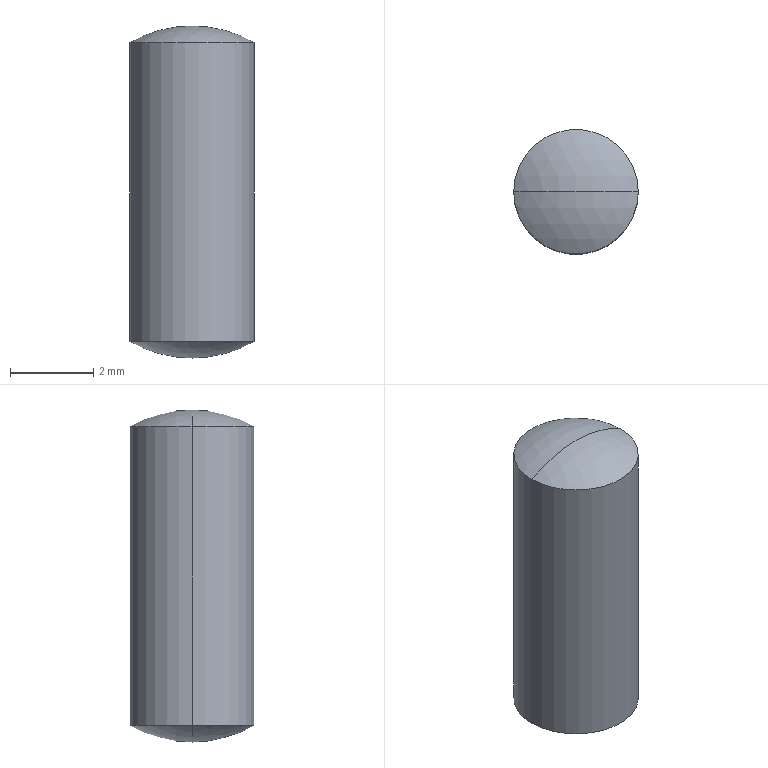Part | SolidWorks | features Attribute 1, Revolution 1 | 1 solid | 6 faces | box 3 x 3 x 8 mm | volume 53.776 mm3 | sphere 4 | cylinder 2 | commonest cylinder face diameters 3 x2
STEP:
#1=CARTESIAN_POINT('',(-1.5,0.,1.598));
#2=VERTEX_POINT('',#1);
#3=CARTESIAN_POINT('',(1.5,0.,1.598));
#4=VERTEX_POINT('',#3);
#5=CARTESIAN_POINT('',(0.,0.,1.598));
#6=DIRECTION('',(0.,0.,-1.));
#7=DIRECTION('',(-1.,0.,0.));
#8=AXIS2_PLACEMENT_3D('',#5,#6,#7);
#9=CIRCLE('',#8,1.5);
#10=EDGE_CURVE('',#2,#4,#9,.T.);
#11=ORIENTED_EDGE('',*,*,#10,.T.);
#12=CARTESIAN_POINT('',(1.5,0.,-5.598));
#13=VERTEX_POINT('',#12);
#14=CARTESIAN_POINT('',(1.5,0.,-47.537));
#15=DIRECTION('',(0.,0.,-1.));
#16=VECTOR('',#15,1000.);
#17=LINE('',#14,#16);
#18=EDGE_CURVE('',#4,#13,#17,.T.);
#19=ORIENTED_EDGE('',*,*,#18,.T.);
#20=CARTESIAN_POINT('',(-1.5,0.,-5.598));
#21=VERTEX_POINT('',#20);
#22=CARTESIAN_POINT('',(0.,0.,-5.598));
#23=DIRECTION('',(0.,0.,-1.));
#24=DIRECTION('',(-1.,0.,0.));
#25=AXIS2_PLACEMENT_3D('',#22,#23,#24);
#26=CIRCLE('',#25,1.5);
#27=EDGE_CURVE('',#21,#13,#26,.T.);
#28=ORIENTED_EDGE('',*,*,#27,.F.);
#29=CARTESIAN_POINT('',(-1.5,0.,-47.537));
#30=DIRECTION('',(0.,0.,-1.));
#31=VECTOR('',#30,1000.);
#32=LINE('',#29,#31);
#33=EDGE_CURVE('',#2,#21,#32,.T.);
#34=ORIENTED_EDGE('',*,*,#33,.F.);
#35=EDGE_LOOP('',(#11,#19,#28,#34));
#36=FACE_OUTER_BOUND('',#35,.T.);
#37=CARTESIAN_POINT('',(0.,0.,-47.537));
#38=DIRECTION('',(0.,0.,-1.));
#39=DIRECTION('',(-1.,0.,0.));
#40=AXIS2_PLACEMENT_3D('',#37,#38,#39);
#41=CYLINDRICAL_SURFACE('',#40,1.5);
#42=ADVANCED_FACE('',(#36),#41,.T.);
#43=CARTESIAN_POINT('',(0.,0.,2.));
#44=VERTEX_POINT('',#43);
#45=CARTESIAN_POINT('',(0.,0.,-1.));
#46=DIRECTION('',(0.,1.,0.));
#47=DIRECTION('',(0.,0.,1.));
#48=AXIS2_PLACEMENT_3D('',#45,#46,#47);
#49=CIRCLE('',#48,3.);
#50=EDGE_CURVE('',#44,#4,#49,.T.);
#51=ORIENTED_EDGE('',*,*,#50,.F.);
#52=CARTESIAN_POINT('',(0.,0.,-1.));
#53=DIRECTION('',(0.,-1.,0.));
#54=DIRECTION('',(1.,0.,0.));
#55=AXIS2_PLACEMENT_3D('',#52,#53,#54);
#56=CIRCLE('',#55,3.);
#57=EDGE_CURVE('',#44,#2,#56,.T.);
#58=ORIENTED_EDGE('',*,*,#57,.T.);
#59=CARTESIAN_POINT('',(0.,0.,1.598));
#60=DIRECTION('',(0.,0.,-1.));
#61=DIRECTION('',(-1.,0.,0.));
#62=AXIS2_PLACEMENT_3D('',#59,#60,#61);
#63=CIRCLE('',#62,1.5);
#64=EDGE_CURVE('',#4,#2,#63,.T.);
#65=ORIENTED_EDGE('',*,*,#64,.F.);
#66=EDGE_LOOP('',(#51,#58,#65));
#67=FACE_OUTER_BOUND('',#66,.T.);
#68=CARTESIAN_POINT('',(0.,0.,-1.));
#69=DIRECTION('',(0.,-1.,0.));
#70=DIRECTION('',(1.,0.,0.));
#71=AXIS2_PLACEMENT_3D('',#68,#69,#70);
#72=SPHERICAL_SURFACE('',#71,3.);
#73=ADVANCED_FACE('',(#67),#72,.T.);
#74=ORIENTED_EDGE('',*,*,#27,.T.);
#75=CARTESIAN_POINT('',(0.,0.,-6.));
#76=VERTEX_POINT('',#75);
#77=CARTESIAN_POINT('',(0.,0.,-3.));
#78=DIRECTION('',(0.,1.,0.));
#79=DIRECTION('',(-1.,0.,0.));
#80=AXIS2_PLACEMENT_3D('',#77,#78,#79);
#81=CIRCLE('',#80,3.);
#82=EDGE_CURVE('',#13,#76,#81,.T.);
#83=ORIENTED_EDGE('',*,*,#82,.T.);
#84=CARTESIAN_POINT('',(0.,0.,-3.));
#85=DIRECTION('',(0.,-1.,0.));
#86=DIRECTION('',(0.,0.,-1.));
#87=AXIS2_PLACEMENT_3D('',#84,#85,#86);
#88=CIRCLE('',#87,3.);
#89=EDGE_CURVE('',#21,#76,#88,.T.);
#90=ORIENTED_EDGE('',*,*,#89,.F.);
#91=EDGE_LOOP('',(#74,#83,#90));
#92=FACE_OUTER_BOUND('',#91,.T.);
#93=CARTESIAN_POINT('',(0.,0.,-3.));
#94=DIRECTION('',(0.,1.,0.));
#95=DIRECTION('',(-1.,0.,0.));
#96=AXIS2_PLACEMENT_3D('',#93,#94,#95);
#97=SPHERICAL_SURFACE('',#96,3.);
#98=ADVANCED_FACE('',(#92),#97,.T.);
#99=ORIENTED_EDGE('',*,*,#82,.F.);
#100=CARTESIAN_POINT('',(0.,0.,-5.598));
#101=DIRECTION('',(0.,0.,-1.));
#102=DIRECTION('',(-1.,0.,0.));
#103=AXIS2_PLACEMENT_3D('',#100,#101,#102);
#104=CIRCLE('',#103,1.5);
#105=EDGE_CURVE('',#13,#21,#104,.T.);
#106=ORIENTED_EDGE('',*,*,#105,.T.);
#107=ORIENTED_EDGE('',*,*,#89,.T.);
#108=EDGE_LOOP('',(#99,#106,#107));
#109=FACE_OUTER_BOUND('',#108,.T.);
#110=CARTESIAN_POINT('',(0.,0.,-3.));
#111=DIRECTION('',(0.,1.,0.));
#112=DIRECTION('',(-1.,0.,0.));
#113=AXIS2_PLACEMENT_3D('',#110,#111,#112);
#114=SPHERICAL_SURFACE('',#113,3.);
#115=ADVANCED_FACE('',(#109),#114,.T.);
#116=ORIENTED_EDGE('',*,*,#57,.F.);
#117=ORIENTED_EDGE('',*,*,#50,.T.);
#118=ORIENTED_EDGE('',*,*,#10,.F.);
#119=EDGE_LOOP('',(#116,#117,#118));
#120=FACE_OUTER_BOUND('',#119,.T.);
#121=CARTESIAN_POINT('',(0.,0.,-1.));
#122=DIRECTION('',(0.,-1.,0.));
#123=DIRECTION('',(1.,0.,0.));
#124=AXIS2_PLACEMENT_3D('',#121,#122,#123);
#125=SPHERICAL_SURFACE('',#124,3.);
#126=ADVANCED_FACE('',(#120),#125,.T.);
#127=ORIENTED_EDGE('',*,*,#18,.F.);
#128=ORIENTED_EDGE('',*,*,#64,.T.);
#129=ORIENTED_EDGE('',*,*,#33,.T.);
#130=ORIENTED_EDGE('',*,*,#105,.F.);
#131=EDGE_LOOP('',(#127,#128,#129,#130));
#132=FACE_OUTER_BOUND('',#131,.T.);
#133=CARTESIAN_POINT('',(0.,0.,-47.537));
#134=DIRECTION('',(0.,0.,-1.));
#135=DIRECTION('',(-1.,0.,0.));
#136=AXIS2_PLACEMENT_3D('',#133,#134,#135);
#137=CYLINDRICAL_SURFACE('',#136,1.5);
#138=ADVANCED_FACE('',(#132),#137,.T.);
#139=CLOSED_SHELL('',(#42,#73,#98,#115,#126,#138));
#140=MANIFOLD_SOLID_BREP('',#139);
#141=CARTESIAN_POINT('',(0.,0.,0.));
#142=DIRECTION('',(0.,0.,1.));
#143=DIRECTION('',(1.,0.,0.));
#144=AXIS2_PLACEMENT_3D('',#141,#142,#143);
#145=(LENGTH_UNIT()NAMED_UNIT(*)SI_UNIT(.MILLI.,.METRE.));
#146=UNCERTAINTY_MEASURE_WITH_UNIT(LENGTH_MEASURE(0.00001),#145,'','');
#147=(NAMED_UNIT(*)PLANE_ANGLE_UNIT()SI_UNIT($,.RADIAN.));
#148=(NAMED_UNIT(*)SI_UNIT($,.STERADIAN.)SOLID_ANGLE_UNIT());
#149=(GEOMETRIC_REPRESENTATION_CONTEXT(3)GLOBAL_UNCERTAINTY_ASSIGNED_CONTEXT((#146))GLOBAL_UNIT_ASSIGNED_CONTEXT((#145,#147,#148))REPRESENTATION_CONTEXT('',''));
#150=ADVANCED_BREP_SHAPE_REPRESENTATION('',(#140,#144),#149);